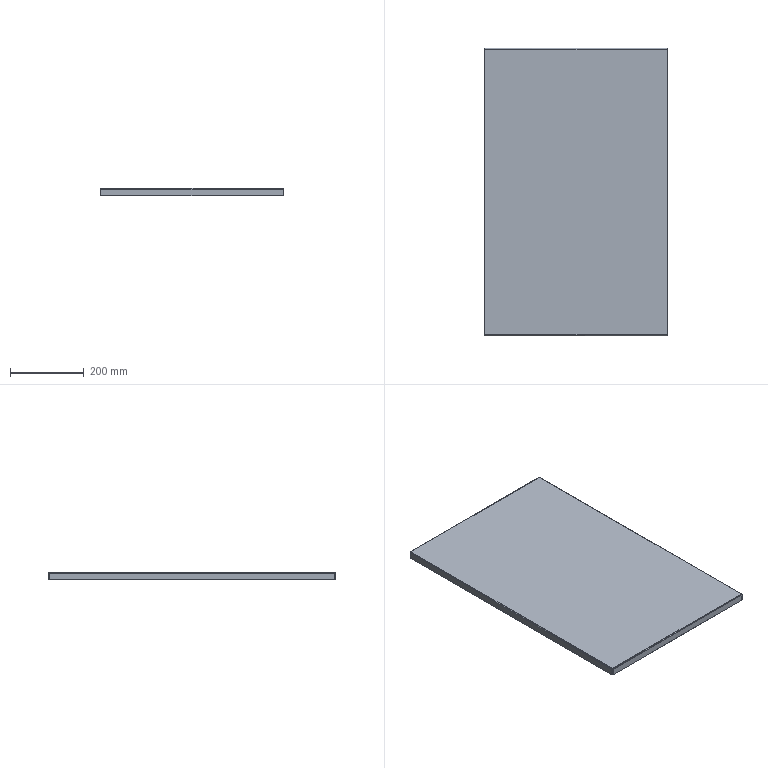Part | STEP file | X77-03017 | 1 solid | 38 faces | box 498 x 778 x 20 mm | volume 649039 mm3 | plane 22 | spline 8 | cylinder 8 | commonest cylinder face diameters 1.473 x4 4.473 x4